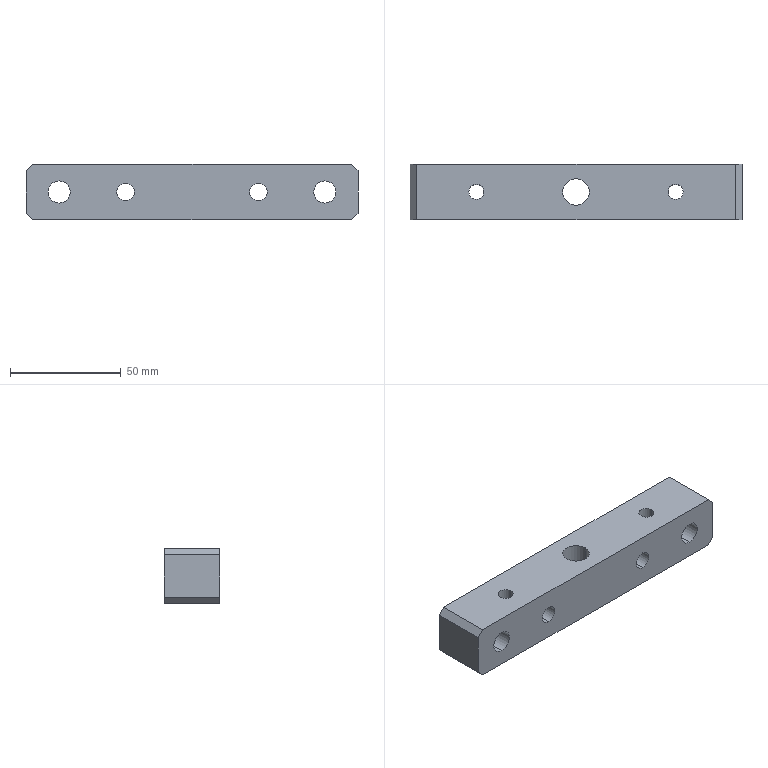Part | STEP file | HXGR200008-05-06 | 1 solid | 24 faces | box 150 x 25 x 25 mm | volume 82216 mm3 | cylinder 14 | plane 10 | commonest cylinder face diameters 6.8 x4 8 x4 10 x4 12 x2
STEP:
#1=CARTESIAN_POINT('',(-30.,-12.5,-4.));
#2=VERTEX_POINT('',#1);
#3=CARTESIAN_POINT('',(-30.,-12.5,4.));
#4=VERTEX_POINT('',#3);
#5=CARTESIAN_POINT('',(-30.,-12.5,0.));
#6=DIRECTION('',(0.,1.,0.));
#7=DIRECTION('',(0.,0.,1.));
#8=AXIS2_PLACEMENT_3D('',#5,#6,#7);
#9=CIRCLE('',#8,4.);
#10=EDGE_CURVE('',#2,#4,#9,.T.);
#11=ORIENTED_EDGE('',*,*,#10,.F.);
#12=CARTESIAN_POINT('',(-30.,12.5,-4.));
#13=VERTEX_POINT('',#12);
#14=CARTESIAN_POINT('',(-30.,12.5,-4.));
#15=DIRECTION('',(0.,1.,0.));
#16=VECTOR('',#15,1000.);
#17=LINE('',#14,#16);
#18=EDGE_CURVE('',#2,#13,#17,.T.);
#19=ORIENTED_EDGE('',*,*,#18,.T.);
#20=CARTESIAN_POINT('',(-30.,12.5,4.));
#21=VERTEX_POINT('',#20);
#22=CARTESIAN_POINT('',(-30.,12.5,0.));
#23=DIRECTION('',(0.,1.,0.));
#24=DIRECTION('',(0.,0.,1.));
#25=AXIS2_PLACEMENT_3D('',#22,#23,#24);
#26=CIRCLE('',#25,4.);
#27=EDGE_CURVE('',#13,#21,#26,.T.);
#28=ORIENTED_EDGE('',*,*,#27,.T.);
#29=CARTESIAN_POINT('',(-30.,12.5,4.));
#30=DIRECTION('',(0.,1.,0.));
#31=VECTOR('',#30,1000.);
#32=LINE('',#29,#31);
#33=EDGE_CURVE('',#4,#21,#32,.T.);
#34=ORIENTED_EDGE('',*,*,#33,.F.);
#35=EDGE_LOOP('',(#11,#19,#28,#34));
#36=FACE_OUTER_BOUND('',#35,.T.);
#37=CARTESIAN_POINT('',(-30.,12.5,0.));
#38=DIRECTION('',(0.,1.,0.));
#39=DIRECTION('',(0.,0.,1.));
#40=AXIS2_PLACEMENT_3D('',#37,#38,#39);
#41=CYLINDRICAL_SURFACE('',#40,4.);
#42=ADVANCED_FACE('',(#36),#41,.F.);
#43=CARTESIAN_POINT('',(30.,-12.5,-4.));
#44=VERTEX_POINT('',#43);
#45=CARTESIAN_POINT('',(30.,-12.5,4.));
#46=VERTEX_POINT('',#45);
#47=CARTESIAN_POINT('',(30.,-12.5,0.));
#48=DIRECTION('',(0.,1.,0.));
#49=DIRECTION('',(0.,0.,1.));
#50=AXIS2_PLACEMENT_3D('',#47,#48,#49);
#51=CIRCLE('',#50,4.);
#52=EDGE_CURVE('',#44,#46,#51,.T.);
#53=ORIENTED_EDGE('',*,*,#52,.F.);
#54=CARTESIAN_POINT('',(30.,12.5,-4.));
#55=VERTEX_POINT('',#54);
#56=CARTESIAN_POINT('',(30.,12.5,-4.));
#57=DIRECTION('',(0.,1.,0.));
#58=VECTOR('',#57,1000.);
#59=LINE('',#56,#58);
#60=EDGE_CURVE('',#44,#55,#59,.T.);
#61=ORIENTED_EDGE('',*,*,#60,.T.);
#62=CARTESIAN_POINT('',(30.,12.5,4.));
#63=VERTEX_POINT('',#62);
#64=CARTESIAN_POINT('',(30.,12.5,0.));
#65=DIRECTION('',(0.,1.,0.));
#66=DIRECTION('',(0.,0.,1.));
#67=AXIS2_PLACEMENT_3D('',#64,#65,#66);
#68=CIRCLE('',#67,4.);
#69=EDGE_CURVE('',#55,#63,#68,.T.);
#70=ORIENTED_EDGE('',*,*,#69,.T.);
#71=CARTESIAN_POINT('',(30.,12.5,4.));
#72=DIRECTION('',(0.,1.,0.));
#73=VECTOR('',#72,1000.);
#74=LINE('',#71,#73);
#75=EDGE_CURVE('',#46,#63,#74,.T.);
#76=ORIENTED_EDGE('',*,*,#75,.F.);
#77=EDGE_LOOP('',(#53,#61,#70,#76));
#78=FACE_OUTER_BOUND('',#77,.T.);
#79=CARTESIAN_POINT('',(30.,12.5,0.));
#80=DIRECTION('',(0.,1.,0.));
#81=DIRECTION('',(0.,0.,1.));
#82=AXIS2_PLACEMENT_3D('',#79,#80,#81);
#83=CYLINDRICAL_SURFACE('',#82,4.);
#84=ADVANCED_FACE('',(#78),#83,.F.);
#85=CARTESIAN_POINT('',(-60.,-12.5,-5.));
#86=VERTEX_POINT('',#85);
#87=CARTESIAN_POINT('',(-60.,-12.5,5.));
#88=VERTEX_POINT('',#87);
#89=CARTESIAN_POINT('',(-60.,-12.5,0.));
#90=DIRECTION('',(0.,1.,0.));
#91=DIRECTION('',(0.,0.,1.));
#92=AXIS2_PLACEMENT_3D('',#89,#90,#91);
#93=CIRCLE('',#92,5.);
#94=EDGE_CURVE('',#86,#88,#93,.T.);
#95=ORIENTED_EDGE('',*,*,#94,.F.);
#96=CARTESIAN_POINT('',(-60.,12.5,-5.));
#97=VERTEX_POINT('',#96);
#98=CARTESIAN_POINT('',(-60.,12.5,-5.));
#99=DIRECTION('',(0.,1.,0.));
#100=VECTOR('',#99,1000.);
#101=LINE('',#98,#100);
#102=EDGE_CURVE('',#86,#97,#101,.T.);
#103=ORIENTED_EDGE('',*,*,#102,.T.);
#104=CARTESIAN_POINT('',(-60.,12.5,5.));
#105=VERTEX_POINT('',#104);
#106=CARTESIAN_POINT('',(-60.,12.5,0.));
#107=DIRECTION('',(0.,1.,0.));
#108=DIRECTION('',(0.,0.,1.));
#109=AXIS2_PLACEMENT_3D('',#106,#107,#108);
#110=CIRCLE('',#109,5.);
#111=EDGE_CURVE('',#97,#105,#110,.T.);
#112=ORIENTED_EDGE('',*,*,#111,.T.);
#113=CARTESIAN_POINT('',(-60.,12.5,5.));
#114=DIRECTION('',(0.,1.,0.));
#115=VECTOR('',#114,1000.);
#116=LINE('',#113,#115);
#117=EDGE_CURVE('',#88,#105,#116,.T.);
#118=ORIENTED_EDGE('',*,*,#117,.F.);
#119=EDGE_LOOP('',(#95,#103,#112,#118));
#120=FACE_OUTER_BOUND('',#119,.T.);
#121=CARTESIAN_POINT('',(-60.,12.5,0.));
#122=DIRECTION('',(0.,1.,0.));
#123=DIRECTION('',(0.,0.,1.));
#124=AXIS2_PLACEMENT_3D('',#121,#122,#123);
#125=CYLINDRICAL_SURFACE('',#124,5.);
#126=ADVANCED_FACE('',(#120),#125,.F.);
#127=CARTESIAN_POINT('',(60.,-12.5,-5.));
#128=VERTEX_POINT('',#127);
#129=CARTESIAN_POINT('',(60.,-12.5,5.));
#130=VERTEX_POINT('',#129);
#131=CARTESIAN_POINT('',(60.,-12.5,0.));
#132=DIRECTION('',(0.,1.,0.));
#133=DIRECTION('',(0.,0.,1.));
#134=AXIS2_PLACEMENT_3D('',#131,#132,#133);
#135=CIRCLE('',#134,5.);
#136=EDGE_CURVE('',#128,#130,#135,.T.);
#137=ORIENTED_EDGE('',*,*,#136,.F.);
#138=CARTESIAN_POINT('',(60.,12.5,-5.));
#139=VERTEX_POINT('',#138);
#140=CARTESIAN_POINT('',(60.,12.5,-5.));
#141=DIRECTION('',(0.,1.,0.));
#142=VECTOR('',#141,1000.);
#143=LINE('',#140,#142);
#144=EDGE_CURVE('',#128,#139,#143,.T.);
#145=ORIENTED_EDGE('',*,*,#144,.T.);
#146=CARTESIAN_POINT('',(60.,12.5,5.));
#147=VERTEX_POINT('',#146);
#148=CARTESIAN_POINT('',(60.,12.5,0.));
#149=DIRECTION('',(0.,1.,0.));
#150=DIRECTION('',(0.,0.,1.));
#151=AXIS2_PLACEMENT_3D('',#148,#149,#150);
#152=CIRCLE('',#151,5.);
#153=EDGE_CURVE('',#139,#147,#152,.T.);
#154=ORIENTED_EDGE('',*,*,#153,.T.);
#155=CARTESIAN_POINT('',(60.,12.5,5.));
#156=DIRECTION('',(0.,1.,0.));
#157=VECTOR('',#156,1000.);
#158=LINE('',#155,#157);
#159=EDGE_CURVE('',#130,#147,#158,.T.);
#160=ORIENTED_EDGE('',*,*,#159,.F.);
#161=EDGE_LOOP('',(#137,#145,#154,#160));
#162=FACE_OUTER_BOUND('',#161,.T.);
#163=CARTESIAN_POINT('',(60.,12.5,0.));
#164=DIRECTION('',(0.,1.,0.));
#165=DIRECTION('',(0.,0.,1.));
#166=AXIS2_PLACEMENT_3D('',#163,#164,#165);
#167=CYLINDRICAL_SURFACE('',#166,5.);
#168=ADVANCED_FACE('',(#162),#167,.F.);
#169=CARTESIAN_POINT('',(-48.4,0.,-12.5));
#170=VERTEX_POINT('',#169);
#171=CARTESIAN_POINT('',(-41.6,0.,-12.5));
#172=VERTEX_POINT('',#171);
#173=CARTESIAN_POINT('',(-45.,0.,-12.5));
#174=DIRECTION('',(0.,0.,1.));
#175=DIRECTION('',(1.,0.,0.));
#176=AXIS2_PLACEMENT_3D('',#173,#174,#175);
#177=CIRCLE('',#176,3.4);
#178=EDGE_CURVE('',#170,#172,#177,.T.);
#179=ORIENTED_EDGE('',*,*,#178,.F.);
#180=CARTESIAN_POINT('',(-48.4,0.,12.5));
#181=VERTEX_POINT('',#180);
#182=CARTESIAN_POINT('',(-48.4,0.,12.5));
#183=DIRECTION('',(0.,0.,1.));
#184=VECTOR('',#183,1000.);
#185=LINE('',#182,#184);
#186=EDGE_CURVE('',#170,#181,#185,.T.);
#187=ORIENTED_EDGE('',*,*,#186,.T.);
#188=CARTESIAN_POINT('',(-41.6,0.,12.5));
#189=VERTEX_POINT('',#188);
#190=CARTESIAN_POINT('',(-45.,0.,12.5));
#191=DIRECTION('',(0.,0.,1.));
#192=DIRECTION('',(1.,0.,0.));
#193=AXIS2_PLACEMENT_3D('',#190,#191,#192);
#194=CIRCLE('',#193,3.4);
#195=EDGE_CURVE('',#181,#189,#194,.T.);
#196=ORIENTED_EDGE('',*,*,#195,.T.);
#197=CARTESIAN_POINT('',(-41.6,0.,12.5));
#198=DIRECTION('',(0.,0.,1.));
#199=VECTOR('',#198,1000.);
#200=LINE('',#197,#199);
#201=EDGE_CURVE('',#172,#189,#200,.T.);
#202=ORIENTED_EDGE('',*,*,#201,.F.);
#203=EDGE_LOOP('',(#179,#187,#196,#202));
#204=FACE_OUTER_BOUND('',#203,.T.);
#205=CARTESIAN_POINT('',(-45.,0.,12.5));
#206=DIRECTION('',(0.,0.,1.));
#207=DIRECTION('',(1.,0.,0.));
#208=AXIS2_PLACEMENT_3D('',#205,#206,#207);
#209=CYLINDRICAL_SURFACE('',#208,3.4);
#210=ADVANCED_FACE('',(#204),#209,.F.);
#211=CARTESIAN_POINT('',(41.6,0.,-12.5));
#212=VERTEX_POINT('',#211);
#213=CARTESIAN_POINT('',(48.4,0.,-12.5));
#214=VERTEX_POINT('',#213);
#215=CARTESIAN_POINT('',(45.,0.,-12.5));
#216=DIRECTION('',(0.,0.,1.));
#217=DIRECTION('',(1.,0.,0.));
#218=AXIS2_PLACEMENT_3D('',#215,#216,#217);
#219=CIRCLE('',#218,3.4);
#220=EDGE_CURVE('',#212,#214,#219,.T.);
#221=ORIENTED_EDGE('',*,*,#220,.F.);
#222=CARTESIAN_POINT('',(41.6,0.,12.5));
#223=VERTEX_POINT('',#222);
#224=CARTESIAN_POINT('',(41.6,0.,12.5));
#225=DIRECTION('',(0.,0.,1.));
#226=VECTOR('',#225,1000.);
#227=LINE('',#224,#226);
#228=EDGE_CURVE('',#212,#223,#227,.T.);
#229=ORIENTED_EDGE('',*,*,#228,.T.);
#230=CARTESIAN_POINT('',(48.4,0.,12.5));
#231=VERTEX_POINT('',#230);
#232=CARTESIAN_POINT('',(45.,0.,12.5));
#233=DIRECTION('',(0.,0.,1.));
#234=DIRECTION('',(1.,0.,0.));
#235=AXIS2_PLACEMENT_3D('',#232,#233,#234);
#236=CIRCLE('',#235,3.4);
#237=EDGE_CURVE('',#223,#231,#236,.T.);
#238=ORIENTED_EDGE('',*,*,#237,.T.);
#239=CARTESIAN_POINT('',(48.4,0.,12.5));
#240=DIRECTION('',(0.,0.,1.));
#241=VECTOR('',#240,1000.);
#242=LINE('',#239,#241);
#243=EDGE_CURVE('',#214,#231,#242,.T.);
#244=ORIENTED_EDGE('',*,*,#243,.F.);
#245=EDGE_LOOP('',(#221,#229,#238,#244));
#246=FACE_OUTER_BOUND('',#245,.T.);
#247=CARTESIAN_POINT('',(45.,0.,12.5));
#248=DIRECTION('',(0.,0.,1.));
#249=DIRECTION('',(1.,0.,0.));
#250=AXIS2_PLACEMENT_3D('',#247,#248,#249);
#251=CYLINDRICAL_SURFACE('',#250,3.4);
#252=ADVANCED_FACE('',(#246),#251,.F.);
#253=CARTESIAN_POINT('',(-6.,0.,-12.5));
#254=VERTEX_POINT('',#253);
#255=CARTESIAN_POINT('',(6.,0.,-12.5));
#256=VERTEX_POINT('',#255);
#257=CARTESIAN_POINT('',(0.,0.,-12.5));
#258=DIRECTION('',(0.,0.,1.));
#259=DIRECTION('',(1.,0.,0.));
#260=AXIS2_PLACEMENT_3D('',#257,#258,#259);
#261=CIRCLE('',#260,6.);
#262=EDGE_CURVE('',#254,#256,#261,.T.);
#263=ORIENTED_EDGE('',*,*,#262,.F.);
#264=CARTESIAN_POINT('',(-6.,0.,12.5));
#265=VERTEX_POINT('',#264);
#266=CARTESIAN_POINT('',(-6.,0.,12.5));
#267=DIRECTION('',(0.,0.,1.));
#268=VECTOR('',#267,1000.);
#269=LINE('',#266,#268);
#270=EDGE_CURVE('',#254,#265,#269,.T.);
#271=ORIENTED_EDGE('',*,*,#270,.T.);
#272=CARTESIAN_POINT('',(6.,0.,12.5));
#273=VERTEX_POINT('',#272);
#274=CARTESIAN_POINT('',(0.,0.,12.5));
#275=DIRECTION('',(0.,0.,1.));
#276=DIRECTION('',(1.,0.,0.));
#277=AXIS2_PLACEMENT_3D('',#274,#275,#276);
#278=CIRCLE('',#277,6.);
#279=EDGE_CURVE('',#265,#273,#278,.T.);
#280=ORIENTED_EDGE('',*,*,#279,.T.);
#281=CARTESIAN_POINT('',(6.,0.,12.5));
#282=DIRECTION('',(0.,0.,1.));
#283=VECTOR('',#282,1000.);
#284=LINE('',#281,#283);
#285=EDGE_CURVE('',#256,#273,#284,.T.);
#286=ORIENTED_EDGE('',*,*,#285,.F.);
#287=EDGE_LOOP('',(#263,#271,#280,#286));
#288=FACE_OUTER_BOUND('',#287,.T.);
#289=CARTESIAN_POINT('',(0.,0.,12.5));
#290=DIRECTION('',(0.,0.,1.));
#291=DIRECTION('',(1.,0.,0.));
#292=AXIS2_PLACEMENT_3D('',#289,#290,#291);
#293=CYLINDRICAL_SURFACE('',#292,6.);
#294=ADVANCED_FACE('',(#288),#293,.F.);
#295=CARTESIAN_POINT('',(-75.,12.5,-9.5));
#296=VERTEX_POINT('',#295);
#297=CARTESIAN_POINT('',(-75.,12.5,9.5));
#298=VERTEX_POINT('',#297);
#299=CARTESIAN_POINT('',(-75.,12.5,12.5));
#300=DIRECTION('',(0.,0.,1.));
#301=VECTOR('',#300,1000.);
#302=LINE('',#299,#301);
#303=EDGE_CURVE('',#296,#298,#302,.T.);
#304=ORIENTED_EDGE('',*,*,#303,.F.);
#305=CARTESIAN_POINT('',(-75.,-12.5,-9.5));
#306=VERTEX_POINT('',#305);
#307=CARTESIAN_POINT('',(-75.,12.5,-9.5));
#308=DIRECTION('',(0.,-1.,0.));
#309=VECTOR('',#308,1000.);
#310=LINE('',#307,#309);
#311=EDGE_CURVE('',#296,#306,#310,.T.);
#312=ORIENTED_EDGE('',*,*,#311,.T.);
#313=CARTESIAN_POINT('',(-75.,-12.5,9.5));
#314=VERTEX_POINT('',#313);
#315=CARTESIAN_POINT('',(-75.,-12.5,12.5));
#316=DIRECTION('',(0.,0.,1.));
#317=VECTOR('',#316,1000.);
#318=LINE('',#315,#317);
#319=EDGE_CURVE('',#306,#314,#318,.T.);
#320=ORIENTED_EDGE('',*,*,#319,.T.);
#321=CARTESIAN_POINT('',(-75.,12.5,9.5));
#322=DIRECTION('',(0.,1.,0.));
#323=VECTOR('',#322,1000.);
#324=LINE('',#321,#323);
#325=EDGE_CURVE('',#314,#298,#324,.T.);
#326=ORIENTED_EDGE('',*,*,#325,.T.);
#327=EDGE_LOOP('',(#304,#312,#320,#326));
#328=FACE_OUTER_BOUND('',#327,.T.);
#329=CARTESIAN_POINT('',(-75.,12.5,12.5));
#330=DIRECTION('',(1.,0.,0.));
#331=DIRECTION('',(0.,0.,-1.));
#332=AXIS2_PLACEMENT_3D('',#329,#330,#331);
#333=PLANE('',#332);
#334=ADVANCED_FACE('',(#328),#333,.F.);
#335=CARTESIAN_POINT('',(-45.,0.,12.5));
#336=DIRECTION('',(0.,0.,1.));
#337=DIRECTION('',(1.,0.,0.));
#338=AXIS2_PLACEMENT_3D('',#335,#336,#337);
#339=CIRCLE('',#338,3.4);
#340=EDGE_CURVE('',#189,#181,#339,.T.);
#341=ORIENTED_EDGE('',*,*,#340,.F.);
#342=ORIENTED_EDGE('',*,*,#195,.F.);
#343=EDGE_LOOP('',(#341,#342));
#344=FACE_BOUND('',#343,.T.);
#345=CARTESIAN_POINT('',(45.,0.,12.5));
#346=DIRECTION('',(0.,0.,1.));
#347=DIRECTION('',(1.,0.,0.));
#348=AXIS2_PLACEMENT_3D('',#345,#346,#347);
#349=CIRCLE('',#348,3.4);
#350=EDGE_CURVE('',#231,#223,#349,.T.);
#351=ORIENTED_EDGE('',*,*,#350,.F.);
#352=ORIENTED_EDGE('',*,*,#237,.F.);
#353=EDGE_LOOP('',(#351,#352));
#354=FACE_BOUND('',#353,.T.);
#355=CARTESIAN_POINT('',(0.,0.,12.5));
#356=DIRECTION('',(0.,0.,1.));
#357=DIRECTION('',(1.,0.,0.));
#358=AXIS2_PLACEMENT_3D('',#355,#356,#357);
#359=CIRCLE('',#358,6.);
#360=EDGE_CURVE('',#273,#265,#359,.T.);
#361=ORIENTED_EDGE('',*,*,#360,.F.);
#362=ORIENTED_EDGE('',*,*,#279,.F.);
#363=EDGE_LOOP('',(#361,#362));
#364=FACE_BOUND('',#363,.T.);
#365=CARTESIAN_POINT('',(-72.,-12.5,12.5));
#366=VERTEX_POINT('',#365);
#367=CARTESIAN_POINT('',(72.,-12.5,12.5));
#368=VERTEX_POINT('',#367);
#369=CARTESIAN_POINT('',(75.,-12.5,12.5));
#370=DIRECTION('',(1.,0.,0.));
#371=VECTOR('',#370,1000.);
#372=LINE('',#369,#371);
#373=EDGE_CURVE('',#366,#368,#372,.T.);
#374=ORIENTED_EDGE('',*,*,#373,.T.);
#375=CARTESIAN_POINT('',(72.,12.5,12.5));
#376=VERTEX_POINT('',#375);
#377=CARTESIAN_POINT('',(72.,12.5,12.5));
#378=DIRECTION('',(0.,1.,0.));
#379=VECTOR('',#378,1000.);
#380=LINE('',#377,#379);
#381=EDGE_CURVE('',#368,#376,#380,.T.);
#382=ORIENTED_EDGE('',*,*,#381,.T.);
#383=CARTESIAN_POINT('',(-72.,12.5,12.5));
#384=VERTEX_POINT('',#383);
#385=CARTESIAN_POINT('',(75.,12.5,12.5));
#386=DIRECTION('',(1.,0.,0.));
#387=VECTOR('',#386,1000.);
#388=LINE('',#385,#387);
#389=EDGE_CURVE('',#384,#376,#388,.T.);
#390=ORIENTED_EDGE('',*,*,#389,.F.);
#391=CARTESIAN_POINT('',(-72.,12.5,12.5));
#392=DIRECTION('',(0.,-1.,0.));
#393=VECTOR('',#392,1000.);
#394=LINE('',#391,#393);
#395=EDGE_CURVE('',#384,#366,#394,.T.);
#396=ORIENTED_EDGE('',*,*,#395,.T.);
#397=EDGE_LOOP('',(#374,#382,#390,#396));
#398=FACE_OUTER_BOUND('',#397,.T.);
#399=CARTESIAN_POINT('',(75.,12.5,12.5));
#400=DIRECTION('',(0.,0.,-1.));
#401=DIRECTION('',(-1.,0.,0.));
#402=AXIS2_PLACEMENT_3D('',#399,#400,#401);
#403=PLANE('',#402);
#404=ADVANCED_FACE('',(#344,#354,#364,#398),#403,.F.);
#405=CARTESIAN_POINT('',(75.,-12.5,9.5));
#406=VERTEX_POINT('',#405);
#407=CARTESIAN_POINT('',(75.,-12.5,-9.5));
#408=VERTEX_POINT('',#407);
#409=CARTESIAN_POINT('',(75.,-12.5,12.5));
#410=DIRECTION('',(0.,0.,-1.));
#411=VECTOR('',#410,1000.);
#412=LINE('',#409,#411);
#413=EDGE_CURVE('',#406,#408,#412,.T.);
#414=ORIENTED_EDGE('',*,*,#413,.T.);
#415=CARTESIAN_POINT('',(75.,12.5,-9.5));
#416=VERTEX_POINT('',#415);
#417=CARTESIAN_POINT('',(75.,12.5,-9.5));
#418=DIRECTION('',(0.,1.,0.));
#419=VECTOR('',#418,1000.);
#420=LINE('',#417,#419);
#421=EDGE_CURVE('',#408,#416,#420,.T.);
#422=ORIENTED_EDGE('',*,*,#421,.T.);
#423=CARTESIAN_POINT('',(75.,12.5,9.5));
#424=VERTEX_POINT('',#423);
#425=CARTESIAN_POINT('',(75.,12.5,12.5));
#426=DIRECTION('',(0.,0.,-1.));
#427=VECTOR('',#426,1000.);
#428=LINE('',#425,#427);
#429=EDGE_CURVE('',#424,#416,#428,.T.);
#430=ORIENTED_EDGE('',*,*,#429,.F.);
#431=CARTESIAN_POINT('',(75.,12.5,9.5));
#432=DIRECTION('',(0.,-1.,0.));
#433=VECTOR('',#432,1000.);
#434=LINE('',#431,#433);
#435=EDGE_CURVE('',#424,#406,#434,.T.);
#436=ORIENTED_EDGE('',*,*,#435,.T.);
#437=EDGE_LOOP('',(#414,#422,#430,#436));
#438=FACE_OUTER_BOUND('',#437,.T.);
#439=CARTESIAN_POINT('',(75.,12.5,12.5));
#440=DIRECTION('',(-1.,0.,0.));
#441=DIRECTION('',(0.,0.,1.));
#442=AXIS2_PLACEMENT_3D('',#439,#440,#441);
#443=PLANE('',#442);
#444=ADVANCED_FACE('',(#438),#443,.F.);
#445=CARTESIAN_POINT('',(-45.,0.,-12.5));
#446=DIRECTION('',(0.,0.,1.));
#447=DIRECTION('',(1.,0.,0.));
#448=AXIS2_PLACEMENT_3D('',#445,#446,#447);
#449=CIRCLE('',#448,3.4);
#450=EDGE_CURVE('',#172,#170,#449,.T.);
#451=ORIENTED_EDGE('',*,*,#450,.T.);
#452=ORIENTED_EDGE('',*,*,#178,.T.);
#453=EDGE_LOOP('',(#451,#452));
#454=FACE_BOUND('',#453,.T.);
#455=CARTESIAN_POINT('',(45.,0.,-12.5));
#456=DIRECTION('',(0.,0.,1.));
#457=DIRECTION('',(1.,0.,0.));
#458=AXIS2_PLACEMENT_3D('',#455,#456,#457);
#459=CIRCLE('',#458,3.4);
#460=EDGE_CURVE('',#214,#212,#459,.T.);
#461=ORIENTED_EDGE('',*,*,#460,.T.);
#462=ORIENTED_EDGE('',*,*,#220,.T.);
#463=EDGE_LOOP('',(#461,#462));
#464=FACE_BOUND('',#463,.T.);
#465=CARTESIAN_POINT('',(0.,0.,-12.5));
#466=DIRECTION('',(0.,0.,1.));
#467=DIRECTION('',(1.,0.,0.));
#468=AXIS2_PLACEMENT_3D('',#465,#466,#467);
#469=CIRCLE('',#468,6.);
#470=EDGE_CURVE('',#256,#254,#469,.T.);
#471=ORIENTED_EDGE('',*,*,#470,.T.);
#472=ORIENTED_EDGE('',*,*,#262,.T.);
#473=EDGE_LOOP('',(#471,#472));
#474=FACE_BOUND('',#473,.T.);
#475=CARTESIAN_POINT('',(72.,12.5,-12.5));
#476=VERTEX_POINT('',#475);
#477=CARTESIAN_POINT('',(-72.,12.5,-12.5));
#478=VERTEX_POINT('',#477);
#479=CARTESIAN_POINT('',(75.,12.5,-12.5));
#480=DIRECTION('',(-1.,0.,0.));
#481=VECTOR('',#480,1000.);
#482=LINE('',#479,#481);
#483=EDGE_CURVE('',#476,#478,#482,.T.);
#484=ORIENTED_EDGE('',*,*,#483,.F.);
#485=CARTESIAN_POINT('',(72.,-12.5,-12.5));
#486=VERTEX_POINT('',#485);
#487=CARTESIAN_POINT('',(72.,12.5,-12.5));
#488=DIRECTION('',(0.,-1.,0.));
#489=VECTOR('',#488,1000.);
#490=LINE('',#487,#489);
#491=EDGE_CURVE('',#476,#486,#490,.T.);
#492=ORIENTED_EDGE('',*,*,#491,.T.);
#493=CARTESIAN_POINT('',(-72.,-12.5,-12.5));
#494=VERTEX_POINT('',#493);
#495=CARTESIAN_POINT('',(75.,-12.5,-12.5));
#496=DIRECTION('',(-1.,0.,0.));
#497=VECTOR('',#496,1000.);
#498=LINE('',#495,#497);
#499=EDGE_CURVE('',#486,#494,#498,.T.);
#500=ORIENTED_EDGE('',*,*,#499,.T.);
#501=CARTESIAN_POINT('',(-72.,12.5,-12.5));
#502=DIRECTION('',(0.,1.,0.));
#503=VECTOR('',#502,1000.);
#504=LINE('',#501,#503);
#505=EDGE_CURVE('',#494,#478,#504,.T.);
#506=ORIENTED_EDGE('',*,*,#505,.T.);
#507=EDGE_LOOP('',(#484,#492,#500,#506));
#508=FACE_OUTER_BOUND('',#507,.T.);
#509=CARTESIAN_POINT('',(75.,12.5,-12.5));
#510=DIRECTION('',(0.,0.,1.));
#511=DIRECTION('',(1.,0.,0.));
#512=AXIS2_PLACEMENT_3D('',#509,#510,#511);
#513=PLANE('',#512);
#514=ADVANCED_FACE('',(#454,#464,#474,#508),#513,.F.);
#515=CARTESIAN_POINT('',(-30.,12.5,0.));
#516=DIRECTION('',(0.,1.,0.));
#517=DIRECTION('',(0.,0.,1.));
#518=AXIS2_PLACEMENT_3D('',#515,#516,#517);
#519=CIRCLE('',#518,4.);
#520=EDGE_CURVE('',#21,#13,#519,.T.);
#521=ORIENTED_EDGE('',*,*,#520,.F.);
#522=ORIENTED_EDGE('',*,*,#27,.F.);
#523=EDGE_LOOP('',(#521,#522));
#524=FACE_BOUND('',#523,.T.);
#525=CARTESIAN_POINT('',(30.,12.5,0.));
#526=DIRECTION('',(0.,1.,0.));
#527=DIRECTION('',(0.,0.,1.));
#528=AXIS2_PLACEMENT_3D('',#525,#526,#527);
#529=CIRCLE('',#528,4.);
#530=EDGE_CURVE('',#63,#55,#529,.T.);
#531=ORIENTED_EDGE('',*,*,#530,.F.);
#532=ORIENTED_EDGE('',*,*,#69,.F.);
#533=EDGE_LOOP('',(#531,#532));
#534=FACE_BOUND('',#533,.T.);
#535=CARTESIAN_POINT('',(-60.,12.5,0.));
#536=DIRECTION('',(0.,1.,0.));
#537=DIRECTION('',(0.,0.,1.));
#538=AXIS2_PLACEMENT_3D('',#535,#536,#537);
#539=CIRCLE('',#538,5.);
#540=EDGE_CURVE('',#105,#97,#539,.T.);
#541=ORIENTED_EDGE('',*,*,#540,.F.);
#542=ORIENTED_EDGE('',*,*,#111,.F.);
#543=EDGE_LOOP('',(#541,#542));
#544=FACE_BOUND('',#543,.T.);
#545=CARTESIAN_POINT('',(60.,12.5,0.));
#546=DIRECTION('',(0.,1.,0.));
#547=DIRECTION('',(0.,0.,1.));
#548=AXIS2_PLACEMENT_3D('',#545,#546,#547);
#549=CIRCLE('',#548,5.);
#550=EDGE_CURVE('',#147,#139,#549,.T.);
#551=ORIENTED_EDGE('',*,*,#550,.F.);
#552=ORIENTED_EDGE('',*,*,#153,.F.);
#553=EDGE_LOOP('',(#551,#552));
#554=FACE_BOUND('',#553,.T.);
#555=ORIENTED_EDGE('',*,*,#429,.T.);
#556=CARTESIAN_POINT('',(42.25,12.5,-42.25));
#557=DIRECTION('',(-0.7071,0.,-0.7071));
#558=VECTOR('',#557,1000.);
#559=LINE('',#556,#558);
#560=EDGE_CURVE('',#416,#476,#559,.T.);
#561=ORIENTED_EDGE('',*,*,#560,.T.);
#562=ORIENTED_EDGE('',*,*,#483,.T.);
#563=CARTESIAN_POINT('',(-42.25,12.5,-42.25));
#564=DIRECTION('',(-0.7071,0.,0.7071));
#565=VECTOR('',#564,1000.);
#566=LINE('',#563,#565);
#567=EDGE_CURVE('',#478,#296,#566,.T.);
#568=ORIENTED_EDGE('',*,*,#567,.T.);
#569=ORIENTED_EDGE('',*,*,#303,.T.);
#570=CARTESIAN_POINT('',(-42.25,12.5,42.25));
#571=DIRECTION('',(0.7071,0.,0.7071));
#572=VECTOR('',#571,1000.);
#573=LINE('',#570,#572);
#574=EDGE_CURVE('',#298,#384,#573,.T.);
#575=ORIENTED_EDGE('',*,*,#574,.T.);
#576=ORIENTED_EDGE('',*,*,#389,.T.);
#577=CARTESIAN_POINT('',(42.25,12.5,42.25));
#578=DIRECTION('',(0.7071,0.,-0.7071));
#579=VECTOR('',#578,1000.);
#580=LINE('',#577,#579);
#581=EDGE_CURVE('',#376,#424,#580,.T.);
#582=ORIENTED_EDGE('',*,*,#581,.T.);
#583=EDGE_LOOP('',(#555,#561,#562,#568,#569,#575,#576,#582));
#584=FACE_OUTER_BOUND('',#583,.T.);
#585=CARTESIAN_POINT('',(0.,12.5,0.));
#586=DIRECTION('',(0.,1.,0.));
#587=DIRECTION('',(0.,0.,1.));
#588=AXIS2_PLACEMENT_3D('',#585,#586,#587);
#589=PLANE('',#588);
#590=ADVANCED_FACE('',(#524,#534,#544,#554,#584),#589,.T.);
#591=CARTESIAN_POINT('',(-30.,-12.5,0.));
#592=DIRECTION('',(0.,1.,0.));
#593=DIRECTION('',(0.,0.,1.));
#594=AXIS2_PLACEMENT_3D('',#591,#592,#593);
#595=CIRCLE('',#594,4.);
#596=EDGE_CURVE('',#4,#2,#595,.T.);
#597=ORIENTED_EDGE('',*,*,#596,.T.);
#598=ORIENTED_EDGE('',*,*,#10,.T.);
#599=EDGE_LOOP('',(#597,#598));
#600=FACE_BOUND('',#599,.T.);
#601=CARTESIAN_POINT('',(30.,-12.5,0.));
#602=DIRECTION('',(0.,1.,0.));
#603=DIRECTION('',(0.,0.,1.));
#604=AXIS2_PLACEMENT_3D('',#601,#602,#603);
#605=CIRCLE('',#604,4.);
#606=EDGE_CURVE('',#46,#44,#605,.T.);
#607=ORIENTED_EDGE('',*,*,#606,.T.);
#608=ORIENTED_EDGE('',*,*,#52,.T.);
#609=EDGE_LOOP('',(#607,#608));
#610=FACE_BOUND('',#609,.T.);
#611=CARTESIAN_POINT('',(-60.,-12.5,0.));
#612=DIRECTION('',(0.,1.,0.));
#613=DIRECTION('',(0.,0.,1.));
#614=AXIS2_PLACEMENT_3D('',#611,#612,#613);
#615=CIRCLE('',#614,5.);
#616=EDGE_CURVE('',#88,#86,#615,.T.);
#617=ORIENTED_EDGE('',*,*,#616,.T.);
#618=ORIENTED_EDGE('',*,*,#94,.T.);
#619=EDGE_LOOP('',(#617,#618));
#620=FACE_BOUND('',#619,.T.);
#621=CARTESIAN_POINT('',(60.,-12.5,0.));
#622=DIRECTION('',(0.,1.,0.));
#623=DIRECTION('',(0.,0.,1.));
#624=AXIS2_PLACEMENT_3D('',#621,#622,#623);
#625=CIRCLE('',#624,5.);
#626=EDGE_CURVE('',#130,#128,#625,.T.);
#627=ORIENTED_EDGE('',*,*,#626,.T.);
#628=ORIENTED_EDGE('',*,*,#136,.T.);
#629=EDGE_LOOP('',(#627,#628));
#630=FACE_BOUND('',#629,.T.);
#631=ORIENTED_EDGE('',*,*,#499,.F.);
#632=CARTESIAN_POINT('',(72.,-12.5,-12.5));
#633=DIRECTION('',(0.7071,0.,0.7071));
#634=VECTOR('',#633,1000.);
#635=LINE('',#632,#634);
#636=EDGE_CURVE('',#486,#408,#635,.T.);
#637=ORIENTED_EDGE('',*,*,#636,.T.);
#638=ORIENTED_EDGE('',*,*,#413,.F.);
#639=CARTESIAN_POINT('',(75.,-12.5,9.5));
#640=DIRECTION('',(-0.7071,0.,0.7071));
#641=VECTOR('',#640,1000.);
#642=LINE('',#639,#641);
#643=EDGE_CURVE('',#406,#368,#642,.T.);
#644=ORIENTED_EDGE('',*,*,#643,.T.);
#645=ORIENTED_EDGE('',*,*,#373,.F.);
#646=CARTESIAN_POINT('',(-72.,-12.5,12.5));
#647=DIRECTION('',(-0.7071,0.,-0.7071));
#648=VECTOR('',#647,1000.);
#649=LINE('',#646,#648);
#650=EDGE_CURVE('',#366,#314,#649,.T.);
#651=ORIENTED_EDGE('',*,*,#650,.T.);
#652=ORIENTED_EDGE('',*,*,#319,.F.);
#653=CARTESIAN_POINT('',(-75.,-12.5,-9.5));
#654=DIRECTION('',(0.7071,0.,-0.7071));
#655=VECTOR('',#654,1000.);
#656=LINE('',#653,#655);
#657=EDGE_CURVE('',#306,#494,#656,.T.);
#658=ORIENTED_EDGE('',*,*,#657,.T.);
#659=EDGE_LOOP('',(#631,#637,#638,#644,#645,#651,#652,#658));
#660=FACE_OUTER_BOUND('',#659,.T.);
#661=CARTESIAN_POINT('',(0.,-12.5,0.));
#662=DIRECTION('',(0.,1.,0.));
#663=DIRECTION('',(0.,0.,1.));
#664=AXIS2_PLACEMENT_3D('',#661,#662,#663);
#665=PLANE('',#664);
#666=ADVANCED_FACE('',(#600,#610,#620,#630,#660),#665,.F.);
#667=ORIENTED_EDGE('',*,*,#270,.F.);
#668=ORIENTED_EDGE('',*,*,#470,.F.);
#669=ORIENTED_EDGE('',*,*,#285,.T.);
#670=ORIENTED_EDGE('',*,*,#360,.T.);
#671=EDGE_LOOP('',(#667,#668,#669,#670));
#672=FACE_OUTER_BOUND('',#671,.T.);
#673=CARTESIAN_POINT('',(0.,0.,12.5));
#674=DIRECTION('',(0.,0.,1.));
#675=DIRECTION('',(1.,0.,0.));
#676=AXIS2_PLACEMENT_3D('',#673,#674,#675);
#677=CYLINDRICAL_SURFACE('',#676,6.);
#678=ADVANCED_FACE('',(#672),#677,.F.);
#679=ORIENTED_EDGE('',*,*,#228,.F.);
#680=ORIENTED_EDGE('',*,*,#460,.F.);
#681=ORIENTED_EDGE('',*,*,#243,.T.);
#682=ORIENTED_EDGE('',*,*,#350,.T.);
#683=EDGE_LOOP('',(#679,#680,#681,#682));
#684=FACE_OUTER_BOUND('',#683,.T.);
#685=CARTESIAN_POINT('',(45.,0.,12.5));
#686=DIRECTION('',(0.,0.,1.));
#687=DIRECTION('',(1.,0.,0.));
#688=AXIS2_PLACEMENT_3D('',#685,#686,#687);
#689=CYLINDRICAL_SURFACE('',#688,3.4);
#690=ADVANCED_FACE('',(#684),#689,.F.);
#691=ORIENTED_EDGE('',*,*,#186,.F.);
#692=ORIENTED_EDGE('',*,*,#450,.F.);
#693=ORIENTED_EDGE('',*,*,#201,.T.);
#694=ORIENTED_EDGE('',*,*,#340,.T.);
#695=EDGE_LOOP('',(#691,#692,#693,#694));
#696=FACE_OUTER_BOUND('',#695,.T.);
#697=CARTESIAN_POINT('',(-45.,0.,12.5));
#698=DIRECTION('',(0.,0.,1.));
#699=DIRECTION('',(1.,0.,0.));
#700=AXIS2_PLACEMENT_3D('',#697,#698,#699);
#701=CYLINDRICAL_SURFACE('',#700,3.4);
#702=ADVANCED_FACE('',(#696),#701,.F.);
#703=ORIENTED_EDGE('',*,*,#144,.F.);
#704=ORIENTED_EDGE('',*,*,#626,.F.);
#705=ORIENTED_EDGE('',*,*,#159,.T.);
#706=ORIENTED_EDGE('',*,*,#550,.T.);
#707=EDGE_LOOP('',(#703,#704,#705,#706));
#708=FACE_OUTER_BOUND('',#707,.T.);
#709=CARTESIAN_POINT('',(60.,12.5,0.));
#710=DIRECTION('',(0.,1.,0.));
#711=DIRECTION('',(0.,0.,1.));
#712=AXIS2_PLACEMENT_3D('',#709,#710,#711);
#713=CYLINDRICAL_SURFACE('',#712,5.);
#714=ADVANCED_FACE('',(#708),#713,.F.);
#715=ORIENTED_EDGE('',*,*,#102,.F.);
#716=ORIENTED_EDGE('',*,*,#616,.F.);
#717=ORIENTED_EDGE('',*,*,#117,.T.);
#718=ORIENTED_EDGE('',*,*,#540,.T.);
#719=EDGE_LOOP('',(#715,#716,#717,#718));
#720=FACE_OUTER_BOUND('',#719,.T.);
#721=CARTESIAN_POINT('',(-60.,12.5,0.));
#722=DIRECTION('',(0.,1.,0.));
#723=DIRECTION('',(0.,0.,1.));
#724=AXIS2_PLACEMENT_3D('',#721,#722,#723);
#725=CYLINDRICAL_SURFACE('',#724,5.);
#726=ADVANCED_FACE('',(#720),#725,.F.);
#727=ORIENTED_EDGE('',*,*,#60,.F.);
#728=ORIENTED_EDGE('',*,*,#606,.F.);
#729=ORIENTED_EDGE('',*,*,#75,.T.);
#730=ORIENTED_EDGE('',*,*,#530,.T.);
#731=EDGE_LOOP('',(#727,#728,#729,#730));
#732=FACE_OUTER_BOUND('',#731,.T.);
#733=CARTESIAN_POINT('',(30.,12.5,0.));
#734=DIRECTION('',(0.,1.,0.));
#735=DIRECTION('',(0.,0.,1.));
#736=AXIS2_PLACEMENT_3D('',#733,#734,#735);
#737=CYLINDRICAL_SURFACE('',#736,4.);
#738=ADVANCED_FACE('',(#732),#737,.F.);
#739=ORIENTED_EDGE('',*,*,#18,.F.);
#740=ORIENTED_EDGE('',*,*,#596,.F.);
#741=ORIENTED_EDGE('',*,*,#33,.T.);
#742=ORIENTED_EDGE('',*,*,#520,.T.);
#743=EDGE_LOOP('',(#739,#740,#741,#742));
#744=FACE_OUTER_BOUND('',#743,.T.);
#745=CARTESIAN_POINT('',(-30.,12.5,0.));
#746=DIRECTION('',(0.,1.,0.));
#747=DIRECTION('',(0.,0.,1.));
#748=AXIS2_PLACEMENT_3D('',#745,#746,#747);
#749=CYLINDRICAL_SURFACE('',#748,4.);
#750=ADVANCED_FACE('',(#744),#749,.F.);
#751=ORIENTED_EDGE('',*,*,#560,.F.);
#752=ORIENTED_EDGE('',*,*,#421,.F.);
#753=ORIENTED_EDGE('',*,*,#636,.F.);
#754=ORIENTED_EDGE('',*,*,#491,.F.);
#755=EDGE_LOOP('',(#751,#752,#753,#754));
#756=FACE_OUTER_BOUND('',#755,.T.);
#757=CARTESIAN_POINT('',(72.,12.5,-12.5));
#758=DIRECTION('',(-0.7071,0.,0.7071));
#759=DIRECTION('',(0.,-1.,0.));
#760=AXIS2_PLACEMENT_3D('',#757,#758,#759);
#761=PLANE('',#760);
#762=ADVANCED_FACE('',(#756),#761,.F.);
#763=ORIENTED_EDGE('',*,*,#581,.F.);
#764=ORIENTED_EDGE('',*,*,#381,.F.);
#765=ORIENTED_EDGE('',*,*,#643,.F.);
#766=ORIENTED_EDGE('',*,*,#435,.F.);
#767=EDGE_LOOP('',(#763,#764,#765,#766));
#768=FACE_OUTER_BOUND('',#767,.T.);
#769=CARTESIAN_POINT('',(75.,12.5,9.5));
#770=DIRECTION('',(-0.7071,0.,-0.7071));
#771=DIRECTION('',(0.,-1.,0.));
#772=AXIS2_PLACEMENT_3D('',#769,#770,#771);
#773=PLANE('',#772);
#774=ADVANCED_FACE('',(#768),#773,.F.);
#775=ORIENTED_EDGE('',*,*,#567,.F.);
#776=ORIENTED_EDGE('',*,*,#505,.F.);
#777=ORIENTED_EDGE('',*,*,#657,.F.);
#778=ORIENTED_EDGE('',*,*,#311,.F.);
#779=EDGE_LOOP('',(#775,#776,#777,#778));
#780=FACE_OUTER_BOUND('',#779,.T.);
#781=CARTESIAN_POINT('',(-75.,12.5,-9.5));
#782=DIRECTION('',(0.7071,0.,0.7071));
#783=DIRECTION('',(0.,-1.,0.));
#784=AXIS2_PLACEMENT_3D('',#781,#782,#783);
#785=PLANE('',#784);
#786=ADVANCED_FACE('',(#780),#785,.F.);
#787=ORIENTED_EDGE('',*,*,#574,.F.);
#788=ORIENTED_EDGE('',*,*,#325,.F.);
#789=ORIENTED_EDGE('',*,*,#650,.F.);
#790=ORIENTED_EDGE('',*,*,#395,.F.);
#791=EDGE_LOOP('',(#787,#788,#789,#790));
#792=FACE_OUTER_BOUND('',#791,.T.);
#793=CARTESIAN_POINT('',(-72.,12.5,12.5));
#794=DIRECTION('',(0.7071,0.,-0.7071));
#795=DIRECTION('',(0.,-1.,0.));
#796=AXIS2_PLACEMENT_3D('',#793,#794,#795);
#797=PLANE('',#796);
#798=ADVANCED_FACE('',(#792),#797,.F.);
#799=CLOSED_SHELL('',(#42,#84,#126,#168,#210,#252,#294,#334,#404,#444,#514,#590,#666,#678,#690,#702,#714,#726,#738,#750,#762,#774,#786,#798));
#800=MANIFOLD_SOLID_BREP('',#799);
#801=CARTESIAN_POINT('',(0.,0.,0.));
#802=DIRECTION('',(0.,0.,1.));
#803=DIRECTION('',(1.,0.,0.));
#804=AXIS2_PLACEMENT_3D('',#801,#802,#803);
#805=(LENGTH_UNIT()NAMED_UNIT(*)SI_UNIT(.MILLI.,.METRE.));
#806=UNCERTAINTY_MEASURE_WITH_UNIT(LENGTH_MEASURE(0.00001),#805,'','');
#807=(NAMED_UNIT(*)PLANE_ANGLE_UNIT()SI_UNIT($,.RADIAN.));
#808=(NAMED_UNIT(*)SI_UNIT($,.STERADIAN.)SOLID_ANGLE_UNIT());
#809=(GEOMETRIC_REPRESENTATION_CONTEXT(3)GLOBAL_UNCERTAINTY_ASSIGNED_CONTEXT((#806))GLOBAL_UNIT_ASSIGNED_CONTEXT((#805,#807,#808))REPRESENTATION_CONTEXT('',''));
#810=ADVANCED_BREP_SHAPE_REPRESENTATION('',(#800,#804),#809);